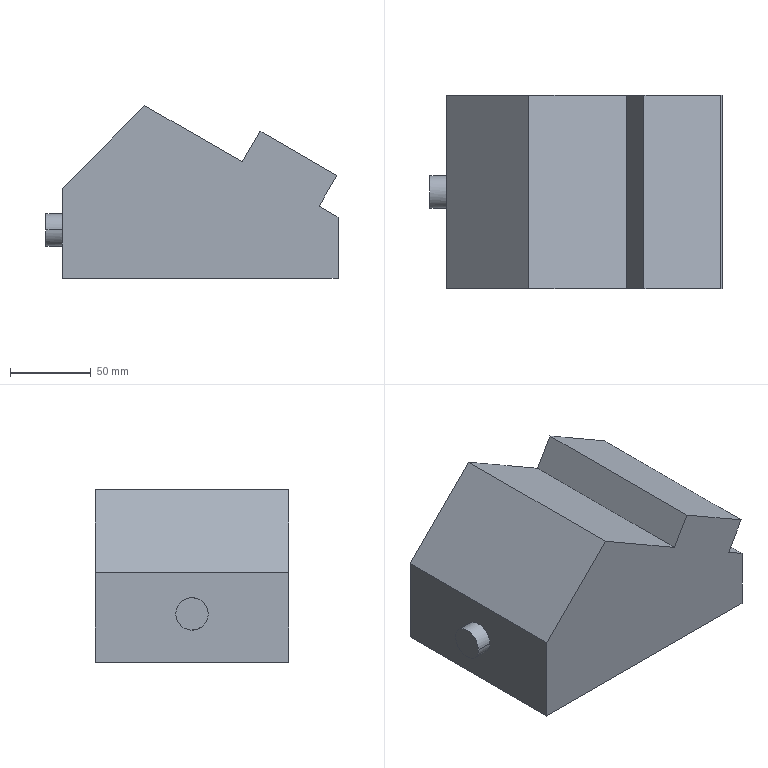Part | NX | features solid 2 | 1 solid | 14 faces | box 181 x 120 x 107 mm | volume 1689782 mm3 | plane 12 | cylinder 2 | commonest cylinder face diameters 20 x2
STEP:
#1=CARTESIAN_POINT('',(-860.736,68.,-205.321));
#2=VERTEX_POINT('',#1);
#3=CARTESIAN_POINT('',(-848.999,68.,-212.097));
#4=VERTEX_POINT('',#3);
#5=CARTESIAN_POINT('',(-860.736,68.,-205.321));
#6=CARTESIAN_POINT('',(-856.824,68.,-207.58));
#7=CARTESIAN_POINT('',(-852.911,68.,-209.838));
#8=CARTESIAN_POINT('',(-848.999,68.,-212.097));
#9=B_SPLINE_CURVE_WITH_KNOTS('',3,(#5,#6,#7,#8),.UNSPECIFIED.,.F.,.F.,(4,4),(0.,1.),.UNSPECIFIED.);
#10=EDGE_CURVE('',#2,#4,#9,.T.);
#11=ORIENTED_EDGE('',*,*,#10,.T.);
#12=CARTESIAN_POINT('',(-848.999,68.,-250.));
#13=VERTEX_POINT('',#12);
#14=CARTESIAN_POINT('',(-848.999,68.,-212.097));
#15=CARTESIAN_POINT('',(-848.999,68.,-224.732));
#16=CARTESIAN_POINT('',(-848.999,68.,-237.366));
#17=CARTESIAN_POINT('',(-848.999,68.,-250.));
#18=B_SPLINE_CURVE_WITH_KNOTS('',3,(#14,#15,#16,#17),.UNSPECIFIED.,.F.,.F.,(4,4),(0.,1.),.UNSPECIFIED.);
#19=EDGE_CURVE('',#4,#13,#18,.T.);
#20=ORIENTED_EDGE('',*,*,#19,.T.);
#21=CARTESIAN_POINT('',(-1019.999,68.,-250.));
#22=VERTEX_POINT('',#21);
#23=CARTESIAN_POINT('',(-848.999,68.,-250.));
#24=CARTESIAN_POINT('',(-905.999,68.,-250.));
#25=CARTESIAN_POINT('',(-962.999,68.,-250.));
#26=CARTESIAN_POINT('',(-1019.999,68.,-250.));
#27=B_SPLINE_CURVE_WITH_KNOTS('',3,(#23,#24,#25,#26),.UNSPECIFIED.,.F.,.F.,(4,4),(0.,1.),.UNSPECIFIED.);
#28=EDGE_CURVE('',#13,#22,#27,.T.);
#29=ORIENTED_EDGE('',*,*,#28,.T.);
#30=CARTESIAN_POINT('',(-1019.999,68.,-194.32));
#31=VERTEX_POINT('',#30);
#32=CARTESIAN_POINT('',(-1019.999,68.,-250.));
#33=CARTESIAN_POINT('',(-1019.999,68.,-231.44));
#34=CARTESIAN_POINT('',(-1019.999,68.,-212.88));
#35=CARTESIAN_POINT('',(-1019.999,68.,-194.32));
#36=B_SPLINE_CURVE_WITH_KNOTS('',3,(#32,#33,#34,#35),.UNSPECIFIED.,.F.,.F.,(4,4),(0.,1.),.UNSPECIFIED.);
#37=EDGE_CURVE('',#22,#31,#36,.T.);
#38=ORIENTED_EDGE('',*,*,#37,.T.);
#39=CARTESIAN_POINT('',(-968.679,68.,-143.));
#40=VERTEX_POINT('',#39);
#41=CARTESIAN_POINT('',(-1019.999,68.,-194.32));
#42=CARTESIAN_POINT('',(-1002.892,68.,-177.213));
#43=CARTESIAN_POINT('',(-985.786,68.,-160.107));
#44=CARTESIAN_POINT('',(-968.679,68.,-143.));
#45=B_SPLINE_CURVE_WITH_KNOTS('',3,(#41,#42,#43,#44),.UNSPECIFIED.,.F.,.F.,(4,4),(0.,1.),.UNSPECIFIED.);
#46=EDGE_CURVE('',#31,#40,#45,.T.);
#47=ORIENTED_EDGE('',*,*,#46,.T.);
#48=CARTESIAN_POINT('',(-908.368,68.,-177.821));
#49=VERTEX_POINT('',#48);
#50=CARTESIAN_POINT('',(-968.679,68.,-143.));
#51=CARTESIAN_POINT('',(-948.575,68.,-154.607));
#52=CARTESIAN_POINT('',(-928.471,68.,-166.214));
#53=CARTESIAN_POINT('',(-908.368,68.,-177.821));
#54=B_SPLINE_CURVE_WITH_KNOTS('',3,(#50,#51,#52,#53),.UNSPECIFIED.,.F.,.F.,(4,4),(0.,1.),.UNSPECIFIED.);
#55=EDGE_CURVE('',#40,#49,#54,.T.);
#56=ORIENTED_EDGE('',*,*,#55,.T.);
#57=CARTESIAN_POINT('',(-897.368,68.,-158.768));
#58=VERTEX_POINT('',#57);
#59=CARTESIAN_POINT('',(-908.368,68.,-177.821));
#60=CARTESIAN_POINT('',(-904.701,68.,-171.47));
#61=CARTESIAN_POINT('',(-901.034,68.,-165.119));
#62=CARTESIAN_POINT('',(-897.368,68.,-158.768));
#63=B_SPLINE_CURVE_WITH_KNOTS('',3,(#59,#60,#61,#62),.UNSPECIFIED.,.F.,.F.,(4,4),(0.,1.),.UNSPECIFIED.);
#64=EDGE_CURVE('',#49,#58,#63,.T.);
#65=ORIENTED_EDGE('',*,*,#64,.T.);
#66=CARTESIAN_POINT('',(-849.736,68.,-186.268));
#67=VERTEX_POINT('',#66);
#68=CARTESIAN_POINT('',(-897.368,68.,-158.768));
#69=CARTESIAN_POINT('',(-881.49,68.,-167.935));
#70=CARTESIAN_POINT('',(-865.613,68.,-177.102));
#71=CARTESIAN_POINT('',(-849.736,68.,-186.268));
#72=B_SPLINE_CURVE_WITH_KNOTS('',3,(#68,#69,#70,#71),.UNSPECIFIED.,.F.,.F.,(4,4),(0.,1.),.UNSPECIFIED.);
#73=EDGE_CURVE('',#58,#67,#72,.T.);
#74=ORIENTED_EDGE('',*,*,#73,.T.);
#75=CARTESIAN_POINT('',(-849.736,68.,-186.268));
#76=CARTESIAN_POINT('',(-853.403,68.,-192.619));
#77=CARTESIAN_POINT('',(-857.07,68.,-198.97));
#78=CARTESIAN_POINT('',(-860.736,68.,-205.321));
#79=B_SPLINE_CURVE_WITH_KNOTS('',3,(#75,#76,#77,#78),.UNSPECIFIED.,.F.,.F.,(4,4),(0.,1.),.UNSPECIFIED.);
#80=EDGE_CURVE('',#67,#2,#79,.T.);
#81=ORIENTED_EDGE('',*,*,#80,.T.);
#82=EDGE_LOOP('',(#11,#20,#29,#38,#47,#56,#65,#74,#81));
#83=FACE_BOUND('',#82,.T.);
#84=CARTESIAN_POINT('',(-934.499,68.,-196.5));
#85=DIRECTION('',(0.,1.,0.));
#86=DIRECTION('',(-1.,0.,0.));
#87=AXIS2_PLACEMENT_3D('',#84,#85,#86);
#88=PLANE('',#87);
#89=ADVANCED_FACE('',(#83),#88,.T.);
#90=ORIENTED_EDGE('',*,*,#19,.F.);
#91=CARTESIAN_POINT('',(-848.999,-52.,-212.097));
#92=VERTEX_POINT('',#91);
#93=CARTESIAN_POINT('',(-848.999,68.,-212.097));
#94=CARTESIAN_POINT('',(-848.999,28.,-212.097));
#95=CARTESIAN_POINT('',(-848.999,-12.,-212.097));
#96=CARTESIAN_POINT('',(-848.999,-52.,-212.097));
#97=B_SPLINE_CURVE_WITH_KNOTS('',3,(#93,#94,#95,#96),.UNSPECIFIED.,.F.,.F.,(4,4),(0.,1.),.UNSPECIFIED.);
#98=EDGE_CURVE('',#4,#92,#97,.T.);
#99=ORIENTED_EDGE('',*,*,#98,.T.);
#100=CARTESIAN_POINT('',(-848.999,-52.,-250.));
#101=VERTEX_POINT('',#100);
#102=CARTESIAN_POINT('',(-848.999,-52.,-212.097));
#103=CARTESIAN_POINT('',(-848.999,-52.,-224.732));
#104=CARTESIAN_POINT('',(-848.999,-52.,-237.366));
#105=CARTESIAN_POINT('',(-848.999,-52.,-250.));
#106=B_SPLINE_CURVE_WITH_KNOTS('',3,(#102,#103,#104,#105),.UNSPECIFIED.,.F.,.F.,(4,4),(0.,1.),.UNSPECIFIED.);
#107=EDGE_CURVE('',#92,#101,#106,.T.);
#108=ORIENTED_EDGE('',*,*,#107,.T.);
#109=CARTESIAN_POINT('',(-848.999,-52.,-250.));
#110=CARTESIAN_POINT('',(-848.999,-12.,-250.));
#111=CARTESIAN_POINT('',(-848.999,28.,-250.));
#112=CARTESIAN_POINT('',(-848.999,68.,-250.));
#113=B_SPLINE_CURVE_WITH_KNOTS('',3,(#109,#110,#111,#112),.UNSPECIFIED.,.F.,.F.,(4,4),(0.,1.),.UNSPECIFIED.);
#114=EDGE_CURVE('',#101,#13,#113,.T.);
#115=ORIENTED_EDGE('',*,*,#114,.T.);
#116=EDGE_LOOP('',(#90,#99,#108,#115));
#117=FACE_BOUND('',#116,.T.);
#118=CARTESIAN_POINT('',(-848.999,8.,-231.049));
#119=DIRECTION('',(1.,0.,0.));
#120=DIRECTION('',(0.,1.,0.));
#121=AXIS2_PLACEMENT_3D('',#118,#119,#120);
#122=PLANE('',#121);
#123=ADVANCED_FACE('',(#117),#122,.T.);
#124=ORIENTED_EDGE('',*,*,#98,.F.);
#125=ORIENTED_EDGE('',*,*,#10,.F.);
#126=CARTESIAN_POINT('',(-860.736,-52.,-205.321));
#127=VERTEX_POINT('',#126);
#128=CARTESIAN_POINT('',(-860.736,68.,-205.321));
#129=CARTESIAN_POINT('',(-860.736,28.,-205.321));
#130=CARTESIAN_POINT('',(-860.736,-12.,-205.321));
#131=CARTESIAN_POINT('',(-860.736,-52.,-205.321));
#132=B_SPLINE_CURVE_WITH_KNOTS('',3,(#128,#129,#130,#131),.UNSPECIFIED.,.F.,.F.,(4,4),(0.,1.),.UNSPECIFIED.);
#133=EDGE_CURVE('',#2,#127,#132,.T.);
#134=ORIENTED_EDGE('',*,*,#133,.T.);
#135=CARTESIAN_POINT('',(-860.736,-52.,-205.321));
#136=CARTESIAN_POINT('',(-856.824,-52.,-207.58));
#137=CARTESIAN_POINT('',(-852.911,-52.,-209.838));
#138=CARTESIAN_POINT('',(-848.999,-52.,-212.097));
#139=B_SPLINE_CURVE_WITH_KNOTS('',3,(#135,#136,#137,#138),.UNSPECIFIED.,.F.,.F.,(4,4),(0.,1.),.UNSPECIFIED.);
#140=EDGE_CURVE('',#127,#92,#139,.T.);
#141=ORIENTED_EDGE('',*,*,#140,.T.);
#142=EDGE_LOOP('',(#124,#125,#134,#141));
#143=FACE_BOUND('',#142,.T.);
#144=CARTESIAN_POINT('',(-854.868,8.,-208.709));
#145=DIRECTION('',(0.5,0.,0.866));
#146=DIRECTION('',(-0.866,0.,0.5));
#147=AXIS2_PLACEMENT_3D('',#144,#145,#146);
#148=PLANE('',#147);
#149=ADVANCED_FACE('',(#143),#148,.T.);
#150=ORIENTED_EDGE('',*,*,#80,.F.);
#151=CARTESIAN_POINT('',(-849.736,-52.,-186.268));
#152=VERTEX_POINT('',#151);
#153=CARTESIAN_POINT('',(-849.736,68.,-186.268));
#154=CARTESIAN_POINT('',(-849.736,28.,-186.268));
#155=CARTESIAN_POINT('',(-849.736,-12.,-186.268));
#156=CARTESIAN_POINT('',(-849.736,-52.,-186.268));
#157=B_SPLINE_CURVE_WITH_KNOTS('',3,(#153,#154,#155,#156),.UNSPECIFIED.,.F.,.F.,(4,4),(0.,1.),.UNSPECIFIED.);
#158=EDGE_CURVE('',#67,#152,#157,.T.);
#159=ORIENTED_EDGE('',*,*,#158,.T.);
#160=CARTESIAN_POINT('',(-849.736,-52.,-186.268));
#161=CARTESIAN_POINT('',(-853.403,-52.,-192.619));
#162=CARTESIAN_POINT('',(-857.07,-52.,-198.97));
#163=CARTESIAN_POINT('',(-860.736,-52.,-205.321));
#164=B_SPLINE_CURVE_WITH_KNOTS('',3,(#160,#161,#162,#163),.UNSPECIFIED.,.F.,.F.,(4,4),(0.,1.),.UNSPECIFIED.);
#165=EDGE_CURVE('',#152,#127,#164,.T.);
#166=ORIENTED_EDGE('',*,*,#165,.T.);
#167=ORIENTED_EDGE('',*,*,#133,.F.);
#168=EDGE_LOOP('',(#150,#159,#166,#167));
#169=FACE_BOUND('',#168,.T.);
#170=CARTESIAN_POINT('',(-855.236,8.,-195.795));
#171=DIRECTION('',(0.866,0.,-0.5));
#172=DIRECTION('',(0.5,0.,0.866));
#173=AXIS2_PLACEMENT_3D('',#170,#171,#172);
#174=PLANE('',#173);
#175=ADVANCED_FACE('',(#169),#174,.T.);
#176=ORIENTED_EDGE('',*,*,#73,.F.);
#177=CARTESIAN_POINT('',(-897.368,-52.,-158.768));
#178=VERTEX_POINT('',#177);
#179=CARTESIAN_POINT('',(-897.368,68.,-158.768));
#180=CARTESIAN_POINT('',(-897.368,28.,-158.768));
#181=CARTESIAN_POINT('',(-897.368,-12.,-158.768));
#182=CARTESIAN_POINT('',(-897.368,-52.,-158.768));
#183=B_SPLINE_CURVE_WITH_KNOTS('',3,(#179,#180,#181,#182),.UNSPECIFIED.,.F.,.F.,(4,4),(0.,1.),.UNSPECIFIED.);
#184=EDGE_CURVE('',#58,#178,#183,.T.);
#185=ORIENTED_EDGE('',*,*,#184,.T.);
#186=CARTESIAN_POINT('',(-897.368,-52.,-158.768));
#187=CARTESIAN_POINT('',(-881.49,-52.,-167.935));
#188=CARTESIAN_POINT('',(-865.613,-52.,-177.102));
#189=CARTESIAN_POINT('',(-849.736,-52.,-186.268));
#190=B_SPLINE_CURVE_WITH_KNOTS('',3,(#186,#187,#188,#189),.UNSPECIFIED.,.F.,.F.,(4,4),(0.,1.),.UNSPECIFIED.);
#191=EDGE_CURVE('',#178,#152,#190,.T.);
#192=ORIENTED_EDGE('',*,*,#191,.T.);
#193=ORIENTED_EDGE('',*,*,#158,.F.);
#194=EDGE_LOOP('',(#176,#185,#192,#193));
#195=FACE_BOUND('',#194,.T.);
#196=CARTESIAN_POINT('',(-873.552,8.,-172.518));
#197=DIRECTION('',(0.5,0.,0.866));
#198=DIRECTION('',(-0.866,0.,0.5));
#199=AXIS2_PLACEMENT_3D('',#196,#197,#198);
#200=PLANE('',#199);
#201=ADVANCED_FACE('',(#195),#200,.T.);
#202=ORIENTED_EDGE('',*,*,#64,.F.);
#203=CARTESIAN_POINT('',(-908.368,-52.,-177.821));
#204=VERTEX_POINT('',#203);
#205=CARTESIAN_POINT('',(-908.368,68.,-177.821));
#206=CARTESIAN_POINT('',(-908.368,28.,-177.821));
#207=CARTESIAN_POINT('',(-908.368,-12.,-177.821));
#208=CARTESIAN_POINT('',(-908.368,-52.,-177.821));
#209=B_SPLINE_CURVE_WITH_KNOTS('',3,(#205,#206,#207,#208),.UNSPECIFIED.,.F.,.F.,(4,4),(0.,1.),.UNSPECIFIED.);
#210=EDGE_CURVE('',#49,#204,#209,.T.);
#211=ORIENTED_EDGE('',*,*,#210,.T.);
#212=CARTESIAN_POINT('',(-908.368,-52.,-177.821));
#213=CARTESIAN_POINT('',(-904.701,-52.,-171.47));
#214=CARTESIAN_POINT('',(-901.034,-52.,-165.119));
#215=CARTESIAN_POINT('',(-897.368,-52.,-158.768));
#216=B_SPLINE_CURVE_WITH_KNOTS('',3,(#212,#213,#214,#215),.UNSPECIFIED.,.F.,.F.,(4,4),(0.,1.),.UNSPECIFIED.);
#217=EDGE_CURVE('',#204,#178,#216,.T.);
#218=ORIENTED_EDGE('',*,*,#217,.T.);
#219=ORIENTED_EDGE('',*,*,#184,.F.);
#220=EDGE_LOOP('',(#202,#211,#218,#219));
#221=FACE_BOUND('',#220,.T.);
#222=CARTESIAN_POINT('',(-902.868,8.,-168.295));
#223=DIRECTION('',(-0.866,0.,0.5));
#224=DIRECTION('',(-0.5,0.,-0.866));
#225=AXIS2_PLACEMENT_3D('',#222,#223,#224);
#226=PLANE('',#225);
#227=ADVANCED_FACE('',(#221),#226,.T.);
#228=CARTESIAN_POINT('',(-968.679,-52.,-143.));
#229=VERTEX_POINT('',#228);
#230=CARTESIAN_POINT('',(-968.679,68.,-143.));
#231=CARTESIAN_POINT('',(-968.679,28.,-143.));
#232=CARTESIAN_POINT('',(-968.679,-12.,-143.));
#233=CARTESIAN_POINT('',(-968.679,-52.,-143.));
#234=B_SPLINE_CURVE_WITH_KNOTS('',3,(#230,#231,#232,#233),.UNSPECIFIED.,.F.,.F.,(4,4),(0.,1.),.UNSPECIFIED.);
#235=EDGE_CURVE('',#40,#229,#234,.T.);
#236=ORIENTED_EDGE('',*,*,#235,.T.);
#237=CARTESIAN_POINT('',(-968.679,-52.,-143.));
#238=CARTESIAN_POINT('',(-948.575,-52.,-154.607));
#239=CARTESIAN_POINT('',(-928.471,-52.,-166.214));
#240=CARTESIAN_POINT('',(-908.368,-52.,-177.821));
#241=B_SPLINE_CURVE_WITH_KNOTS('',3,(#237,#238,#239,#240),.UNSPECIFIED.,.F.,.F.,(4,4),(0.,1.),.UNSPECIFIED.);
#242=EDGE_CURVE('',#229,#204,#241,.T.);
#243=ORIENTED_EDGE('',*,*,#242,.T.);
#244=ORIENTED_EDGE('',*,*,#210,.F.);
#245=ORIENTED_EDGE('',*,*,#55,.F.);
#246=EDGE_LOOP('',(#236,#243,#244,#245));
#247=FACE_BOUND('',#246,.T.);
#248=CARTESIAN_POINT('',(-938.523,8.,-160.41));
#249=DIRECTION('',(0.5,0.,0.866));
#250=DIRECTION('',(-0.866,0.,0.5));
#251=AXIS2_PLACEMENT_3D('',#248,#249,#250);
#252=PLANE('',#251);
#253=ADVANCED_FACE('',(#247),#252,.T.);
#254=ORIENTED_EDGE('',*,*,#46,.F.);
#255=CARTESIAN_POINT('',(-1019.999,-52.,-194.32));
#256=VERTEX_POINT('',#255);
#257=CARTESIAN_POINT('',(-1019.999,68.,-194.32));
#258=CARTESIAN_POINT('',(-1019.999,28.,-194.32));
#259=CARTESIAN_POINT('',(-1019.999,-12.,-194.32));
#260=CARTESIAN_POINT('',(-1019.999,-52.,-194.32));
#261=B_SPLINE_CURVE_WITH_KNOTS('',3,(#257,#258,#259,#260),.UNSPECIFIED.,.F.,.F.,(4,4),(0.,1.),.UNSPECIFIED.);
#262=EDGE_CURVE('',#31,#256,#261,.T.);
#263=ORIENTED_EDGE('',*,*,#262,.T.);
#264=CARTESIAN_POINT('',(-1019.999,-52.,-194.32));
#265=CARTESIAN_POINT('',(-1002.892,-52.,-177.213));
#266=CARTESIAN_POINT('',(-985.786,-52.,-160.107));
#267=CARTESIAN_POINT('',(-968.679,-52.,-143.));
#268=B_SPLINE_CURVE_WITH_KNOTS('',3,(#264,#265,#266,#267),.UNSPECIFIED.,.F.,.F.,(4,4),(0.,1.),.UNSPECIFIED.);
#269=EDGE_CURVE('',#256,#229,#268,.T.);
#270=ORIENTED_EDGE('',*,*,#269,.T.);
#271=ORIENTED_EDGE('',*,*,#235,.F.);
#272=EDGE_LOOP('',(#254,#263,#270,#271));
#273=FACE_BOUND('',#272,.T.);
#274=CARTESIAN_POINT('',(-994.339,8.,-168.66));
#275=DIRECTION('',(-0.7071,0.,0.7071));
#276=DIRECTION('',(-0.7071,0.,-0.7071));
#277=AXIS2_PLACEMENT_3D('',#274,#275,#276);
#278=PLANE('',#277);
#279=ADVANCED_FACE('',(#273),#278,.T.);
#280=CARTESIAN_POINT('',(-1019.999,18.,-220.));
#281=VERTEX_POINT('',#280);
#282=CARTESIAN_POINT('',(-1019.999,-2.,-220.));
#283=VERTEX_POINT('',#282);
#284=CARTESIAN_POINT('',(-1019.999,18.,-220.));
#285=CARTESIAN_POINT('',(-1019.999,18.,-217.386));
#286=CARTESIAN_POINT('',(-1019.999,15.836,-212.165));
#287=CARTESIAN_POINT('',(-1019.999,8.,-208.917));
#288=CARTESIAN_POINT('',(-1019.999,0.1639,-212.166));
#289=CARTESIAN_POINT('',(-1019.999,-2.,-217.383));
#290=CARTESIAN_POINT('',(-1019.999,-2.,-220.));
#291=B_SPLINE_CURVE_WITH_KNOTS('',3,(#284,#285,#286,#287,#288,#289,#290),.UNSPECIFIED.,.F.,.F.,(4,1,1,1,4),(0.5,0.625,0.75,0.875,1.),.UNSPECIFIED.);
#292=EDGE_CURVE('',#281,#283,#291,.T.);
#293=ORIENTED_EDGE('',*,*,#292,.T.);
#294=CARTESIAN_POINT('',(-1019.999,-2.,-220.));
#295=CARTESIAN_POINT('',(-1019.999,-2.,-222.617));
#296=CARTESIAN_POINT('',(-1019.999,0.1638,-227.834));
#297=CARTESIAN_POINT('',(-1019.999,8.,-231.083));
#298=CARTESIAN_POINT('',(-1019.999,15.836,-227.833));
#299=CARTESIAN_POINT('',(-1019.999,18.,-222.619));
#300=CARTESIAN_POINT('',(-1019.999,18.,-220.));
#301=B_SPLINE_CURVE_WITH_KNOTS('',3,(#294,#295,#296,#297,#298,#299,#300),.UNSPECIFIED.,.F.,.F.,(4,1,1,1,4),(0.,0.125,0.25,0.375,0.5),.UNSPECIFIED.);
#302=EDGE_CURVE('',#283,#281,#301,.T.);
#303=ORIENTED_EDGE('',*,*,#302,.T.);
#304=EDGE_LOOP('',(#293,#303));
#305=FACE_BOUND('',#304,.T.);
#306=ORIENTED_EDGE('',*,*,#37,.F.);
#307=CARTESIAN_POINT('',(-1019.999,-52.,-250.));
#308=VERTEX_POINT('',#307);
#309=CARTESIAN_POINT('',(-1019.999,68.,-250.));
#310=CARTESIAN_POINT('',(-1019.999,28.,-250.));
#311=CARTESIAN_POINT('',(-1019.999,-12.,-250.));
#312=CARTESIAN_POINT('',(-1019.999,-52.,-250.));
#313=B_SPLINE_CURVE_WITH_KNOTS('',3,(#309,#310,#311,#312),.UNSPECIFIED.,.F.,.F.,(4,4),(0.,1.),.UNSPECIFIED.);
#314=EDGE_CURVE('',#22,#308,#313,.T.);
#315=ORIENTED_EDGE('',*,*,#314,.T.);
#316=CARTESIAN_POINT('',(-1019.999,-52.,-250.));
#317=CARTESIAN_POINT('',(-1019.999,-52.,-231.44));
#318=CARTESIAN_POINT('',(-1019.999,-52.,-212.88));
#319=CARTESIAN_POINT('',(-1019.999,-52.,-194.32));
#320=B_SPLINE_CURVE_WITH_KNOTS('',3,(#316,#317,#318,#319),.UNSPECIFIED.,.F.,.F.,(4,4),(0.,1.),.UNSPECIFIED.);
#321=EDGE_CURVE('',#308,#256,#320,.T.);
#322=ORIENTED_EDGE('',*,*,#321,.T.);
#323=ORIENTED_EDGE('',*,*,#262,.F.);
#324=EDGE_LOOP('',(#306,#315,#322,#323));
#325=FACE_BOUND('',#324,.T.);
#326=CARTESIAN_POINT('',(-1019.999,8.,-222.16));
#327=DIRECTION('',(-1.,0.,0.));
#328=DIRECTION('',(0.,-1.,0.));
#329=AXIS2_PLACEMENT_3D('',#326,#327,#328);
#330=PLANE('',#329);
#331=ADVANCED_FACE('',(#305,#325),#330,.T.);
#332=ORIENTED_EDGE('',*,*,#28,.F.);
#333=ORIENTED_EDGE('',*,*,#114,.F.);
#334=CARTESIAN_POINT('',(-848.999,-52.,-250.));
#335=CARTESIAN_POINT('',(-905.999,-52.,-250.));
#336=CARTESIAN_POINT('',(-962.999,-52.,-250.));
#337=CARTESIAN_POINT('',(-1019.999,-52.,-250.));
#338=B_SPLINE_CURVE_WITH_KNOTS('',3,(#334,#335,#336,#337),.UNSPECIFIED.,.F.,.F.,(4,4),(0.,1.),.UNSPECIFIED.);
#339=EDGE_CURVE('',#101,#308,#338,.T.);
#340=ORIENTED_EDGE('',*,*,#339,.T.);
#341=ORIENTED_EDGE('',*,*,#314,.F.);
#342=EDGE_LOOP('',(#332,#333,#340,#341));
#343=FACE_BOUND('',#342,.T.);
#344=CARTESIAN_POINT('',(-934.499,8.,-250.));
#345=DIRECTION('',(0.,0.,-1.));
#346=DIRECTION('',(0.,1.,0.));
#347=AXIS2_PLACEMENT_3D('',#344,#345,#346);
#348=PLANE('',#347);
#349=ADVANCED_FACE('',(#343),#348,.T.);
#350=ORIENTED_EDGE('',*,*,#217,.F.);
#351=ORIENTED_EDGE('',*,*,#242,.F.);
#352=ORIENTED_EDGE('',*,*,#269,.F.);
#353=ORIENTED_EDGE('',*,*,#321,.F.);
#354=ORIENTED_EDGE('',*,*,#339,.F.);
#355=ORIENTED_EDGE('',*,*,#107,.F.);
#356=ORIENTED_EDGE('',*,*,#140,.F.);
#357=ORIENTED_EDGE('',*,*,#165,.F.);
#358=ORIENTED_EDGE('',*,*,#191,.F.);
#359=EDGE_LOOP('',(#350,#351,#352,#353,#354,#355,#356,#357,#358));
#360=FACE_BOUND('',#359,.T.);
#361=CARTESIAN_POINT('',(-934.499,-52.,-196.5));
#362=DIRECTION('',(0.,-1.,0.));
#363=DIRECTION('',(1.,0.,0.));
#364=AXIS2_PLACEMENT_3D('',#361,#362,#363);
#365=PLANE('',#364);
#366=ADVANCED_FACE('',(#360),#365,.T.);
#367=CARTESIAN_POINT('',(-1029.999,18.,-220.));
#368=VERTEX_POINT('',#367);
#369=CARTESIAN_POINT('',(-1029.999,18.,-220.));
#370=CARTESIAN_POINT('',(-1026.666,18.,-220.));
#371=CARTESIAN_POINT('',(-1023.332,18.,-220.));
#372=CARTESIAN_POINT('',(-1019.999,18.,-220.));
#373=B_SPLINE_CURVE_WITH_KNOTS('',3,(#369,#370,#371,#372),.UNSPECIFIED.,.F.,.F.,(4,4),(0.,1.),.UNSPECIFIED.);
#374=EDGE_CURVE('',#368,#281,#373,.T.);
#375=ORIENTED_EDGE('',*,*,#374,.T.);
#376=ORIENTED_EDGE('',*,*,#302,.F.);
#377=CARTESIAN_POINT('',(-1029.999,-2.,-220.));
#378=VERTEX_POINT('',#377);
#379=CARTESIAN_POINT('',(-1019.999,-2.,-220.));
#380=CARTESIAN_POINT('',(-1023.332,-2.,-220.));
#381=CARTESIAN_POINT('',(-1026.666,-2.,-220.));
#382=CARTESIAN_POINT('',(-1029.999,-2.,-220.));
#383=B_SPLINE_CURVE_WITH_KNOTS('',3,(#379,#380,#381,#382),.UNSPECIFIED.,.F.,.F.,(4,4),(0.,1.),.UNSPECIFIED.);
#384=EDGE_CURVE('',#283,#378,#383,.T.);
#385=ORIENTED_EDGE('',*,*,#384,.T.);
#386=CARTESIAN_POINT('',(-1029.999,18.,-220.));
#387=CARTESIAN_POINT('',(-1029.999,18.,-222.618));
#388=CARTESIAN_POINT('',(-1029.999,15.837,-227.833));
#389=CARTESIAN_POINT('',(-1029.999,7.999,-231.081));
#390=CARTESIAN_POINT('',(-1029.999,0.1694,-227.842));
#391=CARTESIAN_POINT('',(-1029.999,-2.,-222.611));
#392=CARTESIAN_POINT('',(-1029.999,-2.,-220.));
#393=B_SPLINE_CURVE_WITH_KNOTS('',3,(#386,#387,#388,#389,#390,#391,#392),.UNSPECIFIED.,.F.,.F.,(4,1,1,1,4),(0.5,0.625,0.75,0.875,1.),.UNSPECIFIED.);
#394=EDGE_CURVE('',#378,#368,#393,.F.);
#395=ORIENTED_EDGE('',*,*,#394,.T.);
#396=EDGE_LOOP('',(#375,#376,#385,#395));
#397=FACE_BOUND('',#396,.T.);
#398=CARTESIAN_POINT('',(-1027.999,8.,-220.));
#399=DIRECTION('',(-1.,0.,0.));
#400=DIRECTION('',(0.,-1.,0.));
#401=AXIS2_PLACEMENT_3D('',#398,#399,#400);
#402=CYLINDRICAL_SURFACE('',#401,10.);
#403=ADVANCED_FACE('',(#397),#402,.T.);
#404=ORIENTED_EDGE('',*,*,#374,.F.);
#405=CARTESIAN_POINT('',(-1029.999,-2.,-220.));
#406=CARTESIAN_POINT('',(-1029.999,-2.,-217.389));
#407=CARTESIAN_POINT('',(-1029.999,0.1693,-212.157));
#408=CARTESIAN_POINT('',(-1029.999,8.002,-208.919));
#409=CARTESIAN_POINT('',(-1029.999,15.835,-212.166));
#410=CARTESIAN_POINT('',(-1029.999,18.,-217.382));
#411=CARTESIAN_POINT('',(-1029.999,18.,-220.));
#412=B_SPLINE_CURVE_WITH_KNOTS('',3,(#405,#406,#407,#408,#409,#410,#411),.UNSPECIFIED.,.F.,.F.,(4,1,1,1,4),(0.,0.125,0.25,0.375,0.5),.UNSPECIFIED.);
#413=EDGE_CURVE('',#368,#378,#412,.F.);
#414=ORIENTED_EDGE('',*,*,#413,.T.);
#415=ORIENTED_EDGE('',*,*,#384,.F.);
#416=ORIENTED_EDGE('',*,*,#292,.F.);
#417=EDGE_LOOP('',(#404,#414,#415,#416));
#418=FACE_BOUND('',#417,.T.);
#419=CARTESIAN_POINT('',(-1027.999,8.,-220.));
#420=DIRECTION('',(-1.,0.,0.));
#421=DIRECTION('',(0.,-1.,0.));
#422=AXIS2_PLACEMENT_3D('',#419,#420,#421);
#423=CYLINDRICAL_SURFACE('',#422,10.);
#424=ADVANCED_FACE('',(#418),#423,.T.);
#425=ORIENTED_EDGE('',*,*,#413,.F.);
#426=ORIENTED_EDGE('',*,*,#394,.F.);
#427=EDGE_LOOP('',(#425,#426));
#428=FACE_BOUND('',#427,.T.);
#429=CARTESIAN_POINT('',(-1029.999,7.8,-219.9));
#430=DIRECTION('',(-1.,0.,0.));
#431=DIRECTION('',(0.,-1.,0.));
#432=AXIS2_PLACEMENT_3D('',#429,#430,#431);
#433=PLANE('',#432);
#434=ADVANCED_FACE('',(#428),#433,.T.);
#435=CLOSED_SHELL('',(#89,#123,#149,#175,#201,#227,#253,#279,#331,#349,#366,#403,#424,#434));
#436=MANIFOLD_SOLID_BREP('',#435);
#437=(LENGTH_UNIT()NAMED_UNIT(*)SI_UNIT(.MILLI.,.METRE.));
#438=UNCERTAINTY_MEASURE_WITH_UNIT(LENGTH_MEASURE(0.0508),#437,'','');
#439=(NAMED_UNIT(*)PLANE_ANGLE_UNIT()SI_UNIT($,.RADIAN.));
#440=(NAMED_UNIT(*)SI_UNIT($,.STERADIAN.)SOLID_ANGLE_UNIT());
#441=(GEOMETRIC_REPRESENTATION_CONTEXT(3)GLOBAL_UNCERTAINTY_ASSIGNED_CONTEXT((#438))GLOBAL_UNIT_ASSIGNED_CONTEXT((#437,#439,#440))REPRESENTATION_CONTEXT('',''));
#442=ADVANCED_BREP_SHAPE_REPRESENTATION('',(#436),#441);